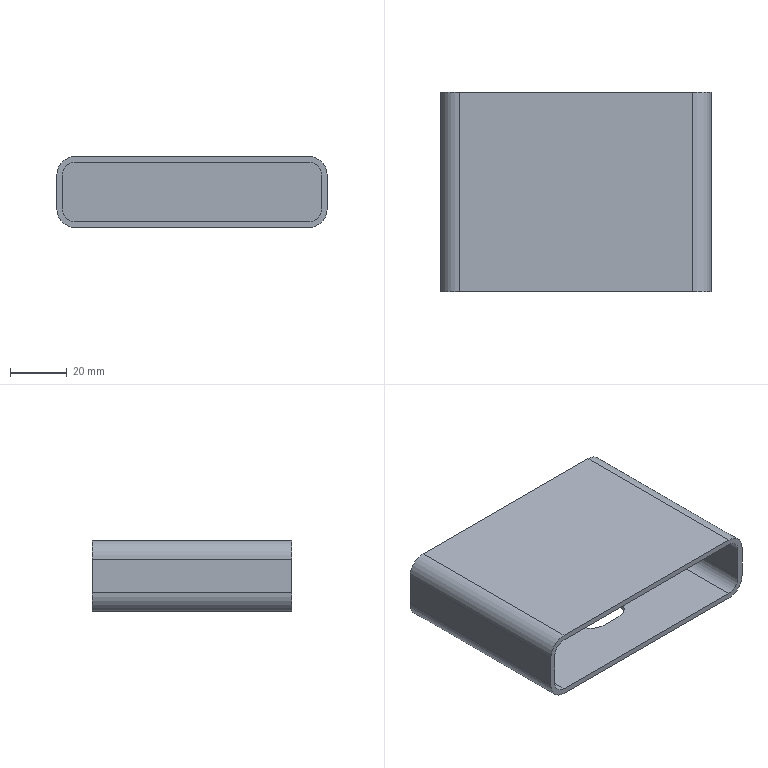Part | STEP file | Guide wheel mechanism revised.sldasm-Part-312 | 1 solid | 24 faces | box 95 x 70 x 25 mm | volume 34478 mm3 | plane 13 | cylinder 11 | commonest cylinder face diameters 9.083 x4 13.083 x4 13 x3
STEP:
#1=CARTESIAN_POINT('',(-10.173,-108.64,-53.));
#2=VERTEX_POINT('',#1);
#3=CARTESIAN_POINT('',(-3.673,-102.14,-53.));
#4=VERTEX_POINT('',#3);
#5=CARTESIAN_POINT('',(-3.673,-108.64,-53.));
#6=DIRECTION('',(0.,0.,-1.));
#7=DIRECTION('',(1.,0.,0.));
#8=AXIS2_PLACEMENT_3D('',#5,#6,#7);
#9=CIRCLE('',#8,6.5);
#10=EDGE_CURVE('',#2,#4,#9,.T.);
#11=ORIENTED_EDGE('',*,*,#10,.F.);
#12=CARTESIAN_POINT('',(-10.173,-108.64,-55.));
#13=VERTEX_POINT('',#12);
#14=CARTESIAN_POINT('',(-10.173,-108.64,0.001));
#15=DIRECTION('',(0.,0.,-1.));
#16=VECTOR('',#15,1000.);
#17=LINE('',#14,#16);
#18=EDGE_CURVE('',#2,#13,#17,.T.);
#19=ORIENTED_EDGE('',*,*,#18,.T.);
#20=CARTESIAN_POINT('',(-3.673,-102.14,-55.));
#21=VERTEX_POINT('',#20);
#22=CARTESIAN_POINT('',(-3.673,-108.64,-55.));
#23=DIRECTION('',(0.,0.,-1.));
#24=DIRECTION('',(-1.,0.,0.));
#25=AXIS2_PLACEMENT_3D('',#22,#23,#24);
#26=CIRCLE('',#25,6.5);
#27=EDGE_CURVE('',#13,#21,#26,.T.);
#28=ORIENTED_EDGE('',*,*,#27,.T.);
#29=CARTESIAN_POINT('',(-3.673,-102.14,0.001));
#30=DIRECTION('',(0.,0.,-1.));
#31=VECTOR('',#30,1000.);
#32=LINE('',#29,#31);
#33=EDGE_CURVE('',#4,#21,#32,.T.);
#34=ORIENTED_EDGE('',*,*,#33,.F.);
#35=EDGE_LOOP('',(#11,#19,#28,#34));
#36=FACE_OUTER_BOUND('',#35,.T.);
#37=CARTESIAN_POINT('',(-3.673,-108.64,0.001));
#38=DIRECTION('',(0.,0.,-1.));
#39=DIRECTION('',(-1.,0.,0.));
#40=AXIS2_PLACEMENT_3D('',#37,#38,#39);
#41=CYLINDRICAL_SURFACE('',#40,6.5);
#42=ADVANCED_FACE('',(#36),#41,.F.);
#43=CARTESIAN_POINT('',(-47.5,-132.5,-48.458));
#44=VERTEX_POINT('',#43);
#45=CARTESIAN_POINT('',(-40.958,-132.5,-55.));
#46=VERTEX_POINT('',#45);
#47=CARTESIAN_POINT('',(-40.958,-132.5,-48.458));
#48=DIRECTION('',(0.,-1.,0.));
#49=DIRECTION('',(0.,0.,1.));
#50=AXIS2_PLACEMENT_3D('',#47,#48,#49);
#51=CIRCLE('',#50,6.542);
#52=EDGE_CURVE('',#44,#46,#51,.T.);
#53=ORIENTED_EDGE('',*,*,#52,.T.);
#54=CARTESIAN_POINT('',(40.958,-132.5,-55.));
#55=VERTEX_POINT('',#54);
#56=CARTESIAN_POINT('',(-40.958,-132.5,-55.));
#57=DIRECTION('',(1.,0.,0.));
#58=VECTOR('',#57,1000.);
#59=LINE('',#56,#58);
#60=EDGE_CURVE('',#46,#55,#59,.T.);
#61=ORIENTED_EDGE('',*,*,#60,.T.);
#62=CARTESIAN_POINT('',(47.5,-132.5,-48.458));
#63=VERTEX_POINT('',#62);
#64=CARTESIAN_POINT('',(40.958,-132.5,-48.458));
#65=DIRECTION('',(0.,-1.,0.));
#66=DIRECTION('',(0.,0.,-1.));
#67=AXIS2_PLACEMENT_3D('',#64,#65,#66);
#68=CIRCLE('',#67,6.542);
#69=EDGE_CURVE('',#55,#63,#68,.T.);
#70=ORIENTED_EDGE('',*,*,#69,.T.);
#71=CARTESIAN_POINT('',(47.5,-132.5,-36.542));
#72=VERTEX_POINT('',#71);
#73=CARTESIAN_POINT('',(47.5,-132.5,-36.542));
#74=DIRECTION('',(0.,0.,1.));
#75=VECTOR('',#74,1000.);
#76=LINE('',#73,#75);
#77=EDGE_CURVE('',#63,#72,#76,.T.);
#78=ORIENTED_EDGE('',*,*,#77,.T.);
#79=CARTESIAN_POINT('',(40.958,-132.5,-30.));
#80=VERTEX_POINT('',#79);
#81=CARTESIAN_POINT('',(40.958,-132.5,-36.542));
#82=DIRECTION('',(0.,-1.,0.));
#83=DIRECTION('',(0.,0.,-1.));
#84=AXIS2_PLACEMENT_3D('',#81,#82,#83);
#85=CIRCLE('',#84,6.542);
#86=EDGE_CURVE('',#72,#80,#85,.T.);
#87=ORIENTED_EDGE('',*,*,#86,.T.);
#88=CARTESIAN_POINT('',(-40.958,-132.5,-30.));
#89=VERTEX_POINT('',#88);
#90=CARTESIAN_POINT('',(-40.958,-132.5,-30.));
#91=DIRECTION('',(-1.,0.,0.));
#92=VECTOR('',#91,1000.);
#93=LINE('',#90,#92);
#94=EDGE_CURVE('',#80,#89,#93,.T.);
#95=ORIENTED_EDGE('',*,*,#94,.T.);
#96=CARTESIAN_POINT('',(-47.5,-132.5,-36.542));
#97=VERTEX_POINT('',#96);
#98=CARTESIAN_POINT('',(-40.958,-132.5,-36.542));
#99=DIRECTION('',(0.,-1.,0.));
#100=DIRECTION('',(0.,0.,1.));
#101=AXIS2_PLACEMENT_3D('',#98,#99,#100);
#102=CIRCLE('',#101,6.542);
#103=EDGE_CURVE('',#89,#97,#102,.T.);
#104=ORIENTED_EDGE('',*,*,#103,.T.);
#105=CARTESIAN_POINT('',(-47.5,-132.5,-36.542));
#106=DIRECTION('',(0.,0.,-1.));
#107=VECTOR('',#106,1000.);
#108=LINE('',#105,#107);
#109=EDGE_CURVE('',#97,#44,#108,.T.);
#110=ORIENTED_EDGE('',*,*,#109,.T.);
#111=EDGE_LOOP('',(#53,#61,#70,#78,#87,#95,#104,#110));
#112=FACE_OUTER_BOUND('',#111,.T.);
#113=CARTESIAN_POINT('',(-45.5,-132.5,-48.458));
#114=VERTEX_POINT('',#113);
#115=CARTESIAN_POINT('',(-40.958,-132.5,-53.));
#116=VERTEX_POINT('',#115);
#117=CARTESIAN_POINT('',(-40.958,-132.5,-48.458));
#118=DIRECTION('',(0.,-1.,0.));
#119=DIRECTION('',(0.,0.,1.));
#120=AXIS2_PLACEMENT_3D('',#117,#118,#119);
#121=CIRCLE('',#120,4.542);
#122=EDGE_CURVE('',#114,#116,#121,.T.);
#123=ORIENTED_EDGE('',*,*,#122,.F.);
#124=CARTESIAN_POINT('',(-45.5,-132.5,-36.542));
#125=VERTEX_POINT('',#124);
#126=CARTESIAN_POINT('',(-45.5,-132.5,-48.458));
#127=DIRECTION('',(0.,0.,-1.));
#128=VECTOR('',#127,1000.);
#129=LINE('',#126,#128);
#130=EDGE_CURVE('',#125,#114,#129,.T.);
#131=ORIENTED_EDGE('',*,*,#130,.F.);
#132=CARTESIAN_POINT('',(-40.958,-132.5,-32.));
#133=VERTEX_POINT('',#132);
#134=CARTESIAN_POINT('',(-40.958,-132.5,-36.542));
#135=DIRECTION('',(0.,-1.,0.));
#136=DIRECTION('',(0.,0.,1.));
#137=AXIS2_PLACEMENT_3D('',#134,#135,#136);
#138=CIRCLE('',#137,4.542);
#139=EDGE_CURVE('',#133,#125,#138,.T.);
#140=ORIENTED_EDGE('',*,*,#139,.F.);
#141=CARTESIAN_POINT('',(40.958,-132.5,-32.));
#142=VERTEX_POINT('',#141);
#143=CARTESIAN_POINT('',(-40.958,-132.5,-32.));
#144=DIRECTION('',(-1.,0.,0.));
#145=VECTOR('',#144,1000.);
#146=LINE('',#143,#145);
#147=EDGE_CURVE('',#142,#133,#146,.T.);
#148=ORIENTED_EDGE('',*,*,#147,.F.);
#149=CARTESIAN_POINT('',(45.5,-132.5,-36.542));
#150=VERTEX_POINT('',#149);
#151=CARTESIAN_POINT('',(40.958,-132.5,-36.542));
#152=DIRECTION('',(0.,-1.,0.));
#153=DIRECTION('',(0.,0.,1.));
#154=AXIS2_PLACEMENT_3D('',#151,#152,#153);
#155=CIRCLE('',#154,4.542);
#156=EDGE_CURVE('',#150,#142,#155,.T.);
#157=ORIENTED_EDGE('',*,*,#156,.F.);
#158=CARTESIAN_POINT('',(45.5,-132.5,-48.458));
#159=VERTEX_POINT('',#158);
#160=CARTESIAN_POINT('',(45.5,-132.5,-48.458));
#161=DIRECTION('',(0.,0.,1.));
#162=VECTOR('',#161,1000.);
#163=LINE('',#160,#162);
#164=EDGE_CURVE('',#159,#150,#163,.T.);
#165=ORIENTED_EDGE('',*,*,#164,.F.);
#166=CARTESIAN_POINT('',(40.958,-132.5,-53.));
#167=VERTEX_POINT('',#166);
#168=CARTESIAN_POINT('',(40.958,-132.5,-48.458));
#169=DIRECTION('',(0.,-1.,0.));
#170=DIRECTION('',(0.,0.,1.));
#171=AXIS2_PLACEMENT_3D('',#168,#169,#170);
#172=CIRCLE('',#171,4.542);
#173=EDGE_CURVE('',#167,#159,#172,.T.);
#174=ORIENTED_EDGE('',*,*,#173,.F.);
#175=CARTESIAN_POINT('',(-40.958,-132.5,-53.));
#176=DIRECTION('',(1.,0.,0.));
#177=VECTOR('',#176,1000.);
#178=LINE('',#175,#177);
#179=EDGE_CURVE('',#116,#167,#178,.T.);
#180=ORIENTED_EDGE('',*,*,#179,.F.);
#181=EDGE_LOOP('',(#123,#131,#140,#148,#157,#165,#174,#180));
#182=FACE_BOUND('',#181,.T.);
#183=CARTESIAN_POINT('',(-40.958,-132.5,-48.458));
#184=DIRECTION('',(0.,1.,0.));
#185=DIRECTION('',(0.,0.,1.));
#186=AXIS2_PLACEMENT_3D('',#183,#184,#185);
#187=PLANE('',#186);
#188=ADVANCED_FACE('',(#112,#182),#187,.F.);
#189=CARTESIAN_POINT('',(-47.5,-62.5,-48.458));
#190=VERTEX_POINT('',#189);
#191=CARTESIAN_POINT('',(-40.958,-62.5,-55.));
#192=VERTEX_POINT('',#191);
#193=CARTESIAN_POINT('',(-40.958,-62.5,-48.458));
#194=DIRECTION('',(0.,-1.,0.));
#195=DIRECTION('',(0.,0.,1.));
#196=AXIS2_PLACEMENT_3D('',#193,#194,#195);
#197=CIRCLE('',#196,6.542);
#198=EDGE_CURVE('',#190,#192,#197,.T.);
#199=ORIENTED_EDGE('',*,*,#198,.T.);
#200=CARTESIAN_POINT('',(-40.958,-132.5,-55.));
#201=DIRECTION('',(0.,1.,0.));
#202=VECTOR('',#201,1000.);
#203=LINE('',#200,#202);
#204=EDGE_CURVE('',#46,#192,#203,.T.);
#205=ORIENTED_EDGE('',*,*,#204,.F.);
#206=ORIENTED_EDGE('',*,*,#52,.F.);
#207=CARTESIAN_POINT('',(-47.5,-132.5,-48.458));
#208=DIRECTION('',(0.,1.,0.));
#209=VECTOR('',#208,1000.);
#210=LINE('',#207,#209);
#211=EDGE_CURVE('',#44,#190,#210,.T.);
#212=ORIENTED_EDGE('',*,*,#211,.T.);
#213=EDGE_LOOP('',(#199,#205,#206,#212));
#214=FACE_OUTER_BOUND('',#213,.T.);
#215=CARTESIAN_POINT('',(-40.958,-132.5,-48.458));
#216=DIRECTION('',(0.,1.,0.));
#217=DIRECTION('',(0.,0.,1.));
#218=AXIS2_PLACEMENT_3D('',#215,#216,#217);
#219=CYLINDRICAL_SURFACE('',#218,6.542);
#220=ADVANCED_FACE('',(#214),#219,.T.);
#221=CARTESIAN_POINT('',(3.673,-115.14,-55.));
#222=VERTEX_POINT('',#221);
#223=CARTESIAN_POINT('',(-3.673,-115.14,-55.));
#224=VERTEX_POINT('',#223);
#225=CARTESIAN_POINT('',(3.673,-115.14,-55.));
#226=DIRECTION('',(-1.,0.,0.));
#227=VECTOR('',#226,1000.);
#228=LINE('',#225,#227);
#229=EDGE_CURVE('',#222,#224,#228,.T.);
#230=ORIENTED_EDGE('',*,*,#229,.F.);
#231=CARTESIAN_POINT('',(3.673,-102.14,-55.));
#232=VERTEX_POINT('',#231);
#233=CARTESIAN_POINT('',(3.673,-108.64,-55.));
#234=DIRECTION('',(0.,0.,-1.));
#235=DIRECTION('',(-1.,0.,0.));
#236=AXIS2_PLACEMENT_3D('',#233,#234,#235);
#237=CIRCLE('',#236,6.5);
#238=EDGE_CURVE('',#232,#222,#237,.T.);
#239=ORIENTED_EDGE('',*,*,#238,.F.);
#240=CARTESIAN_POINT('',(3.673,-102.14,-55.));
#241=DIRECTION('',(1.,0.,0.));
#242=VECTOR('',#241,1000.);
#243=LINE('',#240,#242);
#244=EDGE_CURVE('',#21,#232,#243,.T.);
#245=ORIENTED_EDGE('',*,*,#244,.F.);
#246=ORIENTED_EDGE('',*,*,#27,.F.);
#247=CARTESIAN_POINT('',(-3.673,-108.64,-55.));
#248=DIRECTION('',(0.,0.,-1.));
#249=DIRECTION('',(-1.,0.,0.));
#250=AXIS2_PLACEMENT_3D('',#247,#248,#249);
#251=CIRCLE('',#250,6.5);
#252=EDGE_CURVE('',#224,#13,#251,.T.);
#253=ORIENTED_EDGE('',*,*,#252,.F.);
#254=EDGE_LOOP('',(#230,#239,#245,#246,#253));
#255=FACE_BOUND('',#254,.T.);
#256=CARTESIAN_POINT('',(40.958,-62.5,-55.));
#257=VERTEX_POINT('',#256);
#258=CARTESIAN_POINT('',(-40.958,-62.5,-55.));
#259=DIRECTION('',(1.,0.,0.));
#260=VECTOR('',#259,1000.);
#261=LINE('',#258,#260);
#262=EDGE_CURVE('',#192,#257,#261,.T.);
#263=ORIENTED_EDGE('',*,*,#262,.T.);
#264=CARTESIAN_POINT('',(40.958,-132.5,-55.));
#265=DIRECTION('',(0.,1.,0.));
#266=VECTOR('',#265,1000.);
#267=LINE('',#264,#266);
#268=EDGE_CURVE('',#55,#257,#267,.T.);
#269=ORIENTED_EDGE('',*,*,#268,.F.);
#270=ORIENTED_EDGE('',*,*,#60,.F.);
#271=ORIENTED_EDGE('',*,*,#204,.T.);
#272=EDGE_LOOP('',(#263,#269,#270,#271));
#273=FACE_OUTER_BOUND('',#272,.T.);
#274=CARTESIAN_POINT('',(-40.958,-132.5,-55.));
#275=DIRECTION('',(0.,0.,1.));
#276=DIRECTION('',(1.,0.,0.));
#277=AXIS2_PLACEMENT_3D('',#274,#275,#276);
#278=PLANE('',#277);
#279=ADVANCED_FACE('',(#255,#273),#278,.F.);
#280=CARTESIAN_POINT('',(47.5,-62.5,-48.458));
#281=VERTEX_POINT('',#280);
#282=CARTESIAN_POINT('',(40.958,-62.5,-48.458));
#283=DIRECTION('',(0.,-1.,0.));
#284=DIRECTION('',(0.,0.,-1.));
#285=AXIS2_PLACEMENT_3D('',#282,#283,#284);
#286=CIRCLE('',#285,6.542);
#287=EDGE_CURVE('',#257,#281,#286,.T.);
#288=ORIENTED_EDGE('',*,*,#287,.T.);
#289=CARTESIAN_POINT('',(47.5,-132.5,-48.458));
#290=DIRECTION('',(0.,1.,0.));
#291=VECTOR('',#290,1000.);
#292=LINE('',#289,#291);
#293=EDGE_CURVE('',#63,#281,#292,.T.);
#294=ORIENTED_EDGE('',*,*,#293,.F.);
#295=ORIENTED_EDGE('',*,*,#69,.F.);
#296=ORIENTED_EDGE('',*,*,#268,.T.);
#297=EDGE_LOOP('',(#288,#294,#295,#296));
#298=FACE_OUTER_BOUND('',#297,.T.);
#299=CARTESIAN_POINT('',(40.958,-132.5,-48.458));
#300=DIRECTION('',(0.,1.,0.));
#301=DIRECTION('',(0.,0.,1.));
#302=AXIS2_PLACEMENT_3D('',#299,#300,#301);
#303=CYLINDRICAL_SURFACE('',#302,6.542);
#304=ADVANCED_FACE('',(#298),#303,.T.);
#305=CARTESIAN_POINT('',(47.5,-62.5,-36.542));
#306=VERTEX_POINT('',#305);
#307=CARTESIAN_POINT('',(47.5,-62.5,-36.542));
#308=DIRECTION('',(0.,0.,1.));
#309=VECTOR('',#308,1000.);
#310=LINE('',#307,#309);
#311=EDGE_CURVE('',#281,#306,#310,.T.);
#312=ORIENTED_EDGE('',*,*,#311,.T.);
#313=CARTESIAN_POINT('',(47.5,-132.5,-36.542));
#314=DIRECTION('',(0.,1.,0.));
#315=VECTOR('',#314,1000.);
#316=LINE('',#313,#315);
#317=EDGE_CURVE('',#72,#306,#316,.T.);
#318=ORIENTED_EDGE('',*,*,#317,.F.);
#319=ORIENTED_EDGE('',*,*,#77,.F.);
#320=ORIENTED_EDGE('',*,*,#293,.T.);
#321=EDGE_LOOP('',(#312,#318,#319,#320));
#322=FACE_OUTER_BOUND('',#321,.T.);
#323=CARTESIAN_POINT('',(47.5,-132.5,-36.542));
#324=DIRECTION('',(-1.,0.,0.));
#325=DIRECTION('',(0.,0.,1.));
#326=AXIS2_PLACEMENT_3D('',#323,#324,#325);
#327=PLANE('',#326);
#328=ADVANCED_FACE('',(#322),#327,.F.);
#329=CARTESIAN_POINT('',(40.958,-62.5,-30.));
#330=VERTEX_POINT('',#329);
#331=CARTESIAN_POINT('',(40.958,-62.5,-36.542));
#332=DIRECTION('',(0.,-1.,0.));
#333=DIRECTION('',(0.,0.,-1.));
#334=AXIS2_PLACEMENT_3D('',#331,#332,#333);
#335=CIRCLE('',#334,6.542);
#336=EDGE_CURVE('',#306,#330,#335,.T.);
#337=ORIENTED_EDGE('',*,*,#336,.T.);
#338=CARTESIAN_POINT('',(40.958,-132.5,-30.));
#339=DIRECTION('',(0.,1.,0.));
#340=VECTOR('',#339,1000.);
#341=LINE('',#338,#340);
#342=EDGE_CURVE('',#80,#330,#341,.T.);
#343=ORIENTED_EDGE('',*,*,#342,.F.);
#344=ORIENTED_EDGE('',*,*,#86,.F.);
#345=ORIENTED_EDGE('',*,*,#317,.T.);
#346=EDGE_LOOP('',(#337,#343,#344,#345));
#347=FACE_OUTER_BOUND('',#346,.T.);
#348=CARTESIAN_POINT('',(40.958,-132.5,-36.542));
#349=DIRECTION('',(0.,1.,0.));
#350=DIRECTION('',(0.,0.,1.));
#351=AXIS2_PLACEMENT_3D('',#348,#349,#350);
#352=CYLINDRICAL_SURFACE('',#351,6.542);
#353=ADVANCED_FACE('',(#347),#352,.T.);
#354=CARTESIAN_POINT('',(-40.958,-62.5,-30.));
#355=VERTEX_POINT('',#354);
#356=CARTESIAN_POINT('',(-40.958,-62.5,-30.));
#357=DIRECTION('',(-1.,0.,0.));
#358=VECTOR('',#357,1000.);
#359=LINE('',#356,#358);
#360=EDGE_CURVE('',#330,#355,#359,.T.);
#361=ORIENTED_EDGE('',*,*,#360,.T.);
#362=CARTESIAN_POINT('',(-40.958,-132.5,-30.));
#363=DIRECTION('',(0.,1.,0.));
#364=VECTOR('',#363,1000.);
#365=LINE('',#362,#364);
#366=EDGE_CURVE('',#89,#355,#365,.T.);
#367=ORIENTED_EDGE('',*,*,#366,.F.);
#368=ORIENTED_EDGE('',*,*,#94,.F.);
#369=ORIENTED_EDGE('',*,*,#342,.T.);
#370=EDGE_LOOP('',(#361,#367,#368,#369));
#371=FACE_OUTER_BOUND('',#370,.T.);
#372=CARTESIAN_POINT('',(-40.958,-132.5,-30.));
#373=DIRECTION('',(0.,0.,-1.));
#374=DIRECTION('',(-1.,0.,0.));
#375=AXIS2_PLACEMENT_3D('',#372,#373,#374);
#376=PLANE('',#375);
#377=ADVANCED_FACE('',(#371),#376,.F.);
#378=CARTESIAN_POINT('',(-47.5,-62.5,-36.542));
#379=VERTEX_POINT('',#378);
#380=CARTESIAN_POINT('',(-40.958,-62.5,-36.542));
#381=DIRECTION('',(0.,-1.,0.));
#382=DIRECTION('',(0.,0.,1.));
#383=AXIS2_PLACEMENT_3D('',#380,#381,#382);
#384=CIRCLE('',#383,6.542);
#385=EDGE_CURVE('',#355,#379,#384,.T.);
#386=ORIENTED_EDGE('',*,*,#385,.T.);
#387=CARTESIAN_POINT('',(-47.5,-132.5,-36.542));
#388=DIRECTION('',(0.,1.,0.));
#389=VECTOR('',#388,1000.);
#390=LINE('',#387,#389);
#391=EDGE_CURVE('',#97,#379,#390,.T.);
#392=ORIENTED_EDGE('',*,*,#391,.F.);
#393=ORIENTED_EDGE('',*,*,#103,.F.);
#394=ORIENTED_EDGE('',*,*,#366,.T.);
#395=EDGE_LOOP('',(#386,#392,#393,#394));
#396=FACE_OUTER_BOUND('',#395,.T.);
#397=CARTESIAN_POINT('',(-40.958,-132.5,-36.542));
#398=DIRECTION('',(0.,1.,0.));
#399=DIRECTION('',(0.,0.,1.));
#400=AXIS2_PLACEMENT_3D('',#397,#398,#399);
#401=CYLINDRICAL_SURFACE('',#400,6.542);
#402=ADVANCED_FACE('',(#396),#401,.T.);
#403=CARTESIAN_POINT('',(-47.5,-62.5,-36.542));
#404=DIRECTION('',(0.,0.,-1.));
#405=VECTOR('',#404,1000.);
#406=LINE('',#403,#405);
#407=EDGE_CURVE('',#379,#190,#406,.T.);
#408=ORIENTED_EDGE('',*,*,#407,.T.);
#409=ORIENTED_EDGE('',*,*,#211,.F.);
#410=ORIENTED_EDGE('',*,*,#109,.F.);
#411=ORIENTED_EDGE('',*,*,#391,.T.);
#412=EDGE_LOOP('',(#408,#409,#410,#411));
#413=FACE_OUTER_BOUND('',#412,.T.);
#414=CARTESIAN_POINT('',(-47.5,-132.5,-36.542));
#415=DIRECTION('',(1.,0.,0.));
#416=DIRECTION('',(0.,0.,-1.));
#417=AXIS2_PLACEMENT_3D('',#414,#415,#416);
#418=PLANE('',#417);
#419=ADVANCED_FACE('',(#413),#418,.F.);
#420=ORIENTED_EDGE('',*,*,#198,.F.);
#421=ORIENTED_EDGE('',*,*,#407,.F.);
#422=ORIENTED_EDGE('',*,*,#385,.F.);
#423=ORIENTED_EDGE('',*,*,#360,.F.);
#424=ORIENTED_EDGE('',*,*,#336,.F.);
#425=ORIENTED_EDGE('',*,*,#311,.F.);
#426=ORIENTED_EDGE('',*,*,#287,.F.);
#427=ORIENTED_EDGE('',*,*,#262,.F.);
#428=EDGE_LOOP('',(#420,#421,#422,#423,#424,#425,#426,#427));
#429=FACE_OUTER_BOUND('',#428,.T.);
#430=CARTESIAN_POINT('',(-40.958,-62.5,-48.458));
#431=DIRECTION('',(0.,1.,0.));
#432=DIRECTION('',(0.,0.,1.));
#433=AXIS2_PLACEMENT_3D('',#430,#431,#432);
#434=PLANE('',#433);
#435=ADVANCED_FACE('',(#429),#434,.T.);
#436=CARTESIAN_POINT('',(-45.5,-64.5,-48.458));
#437=VERTEX_POINT('',#436);
#438=CARTESIAN_POINT('',(-40.958,-64.5,-53.));
#439=VERTEX_POINT('',#438);
#440=CARTESIAN_POINT('',(-40.958,-64.5,-48.458));
#441=DIRECTION('',(0.,-1.,0.));
#442=DIRECTION('',(0.,0.,1.));
#443=AXIS2_PLACEMENT_3D('',#440,#441,#442);
#444=CIRCLE('',#443,4.542);
#445=EDGE_CURVE('',#437,#439,#444,.T.);
#446=ORIENTED_EDGE('',*,*,#445,.F.);
#447=CARTESIAN_POINT('',(-45.5,-132.5,-48.458));
#448=DIRECTION('',(0.,1.,0.));
#449=VECTOR('',#448,1000.);
#450=LINE('',#447,#449);
#451=EDGE_CURVE('',#114,#437,#450,.T.);
#452=ORIENTED_EDGE('',*,*,#451,.F.);
#453=ORIENTED_EDGE('',*,*,#122,.T.);
#454=CARTESIAN_POINT('',(-40.958,-132.5,-53.));
#455=DIRECTION('',(0.,1.,0.));
#456=VECTOR('',#455,1000.);
#457=LINE('',#454,#456);
#458=EDGE_CURVE('',#116,#439,#457,.T.);
#459=ORIENTED_EDGE('',*,*,#458,.T.);
#460=EDGE_LOOP('',(#446,#452,#453,#459));
#461=FACE_OUTER_BOUND('',#460,.T.);
#462=CARTESIAN_POINT('',(-40.958,-132.5,-48.458));
#463=DIRECTION('',(0.,1.,0.));
#464=DIRECTION('',(0.,0.,1.));
#465=AXIS2_PLACEMENT_3D('',#462,#463,#464);
#466=CYLINDRICAL_SURFACE('',#465,4.542);
#467=ADVANCED_FACE('',(#461),#466,.F.);
#468=CARTESIAN_POINT('',(3.673,-102.14,-53.));
#469=VERTEX_POINT('',#468);
#470=CARTESIAN_POINT('',(3.673,-115.14,-53.));
#471=VERTEX_POINT('',#470);
#472=CARTESIAN_POINT('',(3.673,-108.64,-53.));
#473=DIRECTION('',(0.,0.,-1.));
#474=DIRECTION('',(1.,0.,0.));
#475=AXIS2_PLACEMENT_3D('',#472,#473,#474);
#476=CIRCLE('',#475,6.5);
#477=EDGE_CURVE('',#469,#471,#476,.T.);
#478=ORIENTED_EDGE('',*,*,#477,.T.);
#479=CARTESIAN_POINT('',(-3.673,-115.14,-53.));
#480=VERTEX_POINT('',#479);
#481=CARTESIAN_POINT('',(3.673,-115.14,-53.));
#482=DIRECTION('',(-1.,0.,0.));
#483=VECTOR('',#482,1000.);
#484=LINE('',#481,#483);
#485=EDGE_CURVE('',#471,#480,#484,.T.);
#486=ORIENTED_EDGE('',*,*,#485,.T.);
#487=CARTESIAN_POINT('',(-3.673,-108.64,-53.));
#488=DIRECTION('',(0.,0.,-1.));
#489=DIRECTION('',(1.,0.,0.));
#490=AXIS2_PLACEMENT_3D('',#487,#488,#489);
#491=CIRCLE('',#490,6.5);
#492=EDGE_CURVE('',#480,#2,#491,.T.);
#493=ORIENTED_EDGE('',*,*,#492,.T.);
#494=ORIENTED_EDGE('',*,*,#10,.T.);
#495=CARTESIAN_POINT('',(3.673,-102.14,-53.));
#496=DIRECTION('',(1.,0.,0.));
#497=VECTOR('',#496,1000.);
#498=LINE('',#495,#497);
#499=EDGE_CURVE('',#4,#469,#498,.T.);
#500=ORIENTED_EDGE('',*,*,#499,.T.);
#501=EDGE_LOOP('',(#478,#486,#493,#494,#500));
#502=FACE_BOUND('',#501,.T.);
#503=CARTESIAN_POINT('',(40.958,-64.5,-53.));
#504=VERTEX_POINT('',#503);
#505=CARTESIAN_POINT('',(-40.958,-64.5,-53.));
#506=DIRECTION('',(1.,0.,0.));
#507=VECTOR('',#506,1000.);
#508=LINE('',#505,#507);
#509=EDGE_CURVE('',#439,#504,#508,.T.);
#510=ORIENTED_EDGE('',*,*,#509,.F.);
#511=ORIENTED_EDGE('',*,*,#458,.F.);
#512=ORIENTED_EDGE('',*,*,#179,.T.);
#513=CARTESIAN_POINT('',(40.958,-132.5,-53.));
#514=DIRECTION('',(0.,1.,0.));
#515=VECTOR('',#514,1000.);
#516=LINE('',#513,#515);
#517=EDGE_CURVE('',#167,#504,#516,.T.);
#518=ORIENTED_EDGE('',*,*,#517,.T.);
#519=EDGE_LOOP('',(#510,#511,#512,#518));
#520=FACE_OUTER_BOUND('',#519,.T.);
#521=CARTESIAN_POINT('',(-40.958,-132.5,-53.));
#522=DIRECTION('',(0.,0.,1.));
#523=DIRECTION('',(1.,0.,0.));
#524=AXIS2_PLACEMENT_3D('',#521,#522,#523);
#525=PLANE('',#524);
#526=ADVANCED_FACE('',(#502,#520),#525,.T.);
#527=CARTESIAN_POINT('',(45.5,-64.5,-48.458));
#528=VERTEX_POINT('',#527);
#529=CARTESIAN_POINT('',(40.958,-64.5,-48.458));
#530=DIRECTION('',(0.,-1.,0.));
#531=DIRECTION('',(0.,0.,1.));
#532=AXIS2_PLACEMENT_3D('',#529,#530,#531);
#533=CIRCLE('',#532,4.542);
#534=EDGE_CURVE('',#504,#528,#533,.T.);
#535=ORIENTED_EDGE('',*,*,#534,.F.);
#536=ORIENTED_EDGE('',*,*,#517,.F.);
#537=ORIENTED_EDGE('',*,*,#173,.T.);
#538=CARTESIAN_POINT('',(45.5,-132.5,-48.458));
#539=DIRECTION('',(0.,1.,0.));
#540=VECTOR('',#539,1000.);
#541=LINE('',#538,#540);
#542=EDGE_CURVE('',#159,#528,#541,.T.);
#543=ORIENTED_EDGE('',*,*,#542,.T.);
#544=EDGE_LOOP('',(#535,#536,#537,#543));
#545=FACE_OUTER_BOUND('',#544,.T.);
#546=CARTESIAN_POINT('',(40.958,-132.5,-48.458));
#547=DIRECTION('',(0.,1.,0.));
#548=DIRECTION('',(0.,0.,1.));
#549=AXIS2_PLACEMENT_3D('',#546,#547,#548);
#550=CYLINDRICAL_SURFACE('',#549,4.542);
#551=ADVANCED_FACE('',(#545),#550,.F.);
#552=CARTESIAN_POINT('',(45.5,-64.5,-36.542));
#553=VERTEX_POINT('',#552);
#554=CARTESIAN_POINT('',(45.5,-64.5,-48.458));
#555=DIRECTION('',(0.,0.,1.));
#556=VECTOR('',#555,1000.);
#557=LINE('',#554,#556);
#558=EDGE_CURVE('',#528,#553,#557,.T.);
#559=ORIENTED_EDGE('',*,*,#558,.F.);
#560=ORIENTED_EDGE('',*,*,#542,.F.);
#561=ORIENTED_EDGE('',*,*,#164,.T.);
#562=CARTESIAN_POINT('',(45.5,-132.5,-36.542));
#563=DIRECTION('',(0.,1.,0.));
#564=VECTOR('',#563,1000.);
#565=LINE('',#562,#564);
#566=EDGE_CURVE('',#150,#553,#565,.T.);
#567=ORIENTED_EDGE('',*,*,#566,.T.);
#568=EDGE_LOOP('',(#559,#560,#561,#567));
#569=FACE_OUTER_BOUND('',#568,.T.);
#570=CARTESIAN_POINT('',(45.5,-132.5,-36.542));
#571=DIRECTION('',(-1.,0.,0.));
#572=DIRECTION('',(0.,0.,1.));
#573=AXIS2_PLACEMENT_3D('',#570,#571,#572);
#574=PLANE('',#573);
#575=ADVANCED_FACE('',(#569),#574,.T.);
#576=CARTESIAN_POINT('',(40.958,-64.5,-32.));
#577=VERTEX_POINT('',#576);
#578=CARTESIAN_POINT('',(40.958,-64.5,-36.542));
#579=DIRECTION('',(0.,-1.,0.));
#580=DIRECTION('',(0.,0.,1.));
#581=AXIS2_PLACEMENT_3D('',#578,#579,#580);
#582=CIRCLE('',#581,4.542);
#583=EDGE_CURVE('',#553,#577,#582,.T.);
#584=ORIENTED_EDGE('',*,*,#583,.F.);
#585=ORIENTED_EDGE('',*,*,#566,.F.);
#586=ORIENTED_EDGE('',*,*,#156,.T.);
#587=CARTESIAN_POINT('',(40.958,-132.5,-32.));
#588=DIRECTION('',(0.,1.,0.));
#589=VECTOR('',#588,1000.);
#590=LINE('',#587,#589);
#591=EDGE_CURVE('',#142,#577,#590,.T.);
#592=ORIENTED_EDGE('',*,*,#591,.T.);
#593=EDGE_LOOP('',(#584,#585,#586,#592));
#594=FACE_OUTER_BOUND('',#593,.T.);
#595=CARTESIAN_POINT('',(40.958,-132.5,-36.542));
#596=DIRECTION('',(0.,1.,0.));
#597=DIRECTION('',(0.,0.,1.));
#598=AXIS2_PLACEMENT_3D('',#595,#596,#597);
#599=CYLINDRICAL_SURFACE('',#598,4.542);
#600=ADVANCED_FACE('',(#594),#599,.F.);
#601=CARTESIAN_POINT('',(-40.958,-64.5,-32.));
#602=VERTEX_POINT('',#601);
#603=CARTESIAN_POINT('',(-40.958,-64.5,-32.));
#604=DIRECTION('',(-1.,0.,0.));
#605=VECTOR('',#604,1000.);
#606=LINE('',#603,#605);
#607=EDGE_CURVE('',#577,#602,#606,.T.);
#608=ORIENTED_EDGE('',*,*,#607,.F.);
#609=ORIENTED_EDGE('',*,*,#591,.F.);
#610=ORIENTED_EDGE('',*,*,#147,.T.);
#611=CARTESIAN_POINT('',(-40.958,-132.5,-32.));
#612=DIRECTION('',(0.,1.,0.));
#613=VECTOR('',#612,1000.);
#614=LINE('',#611,#613);
#615=EDGE_CURVE('',#133,#602,#614,.T.);
#616=ORIENTED_EDGE('',*,*,#615,.T.);
#617=EDGE_LOOP('',(#608,#609,#610,#616));
#618=FACE_OUTER_BOUND('',#617,.T.);
#619=CARTESIAN_POINT('',(-40.958,-132.5,-32.));
#620=DIRECTION('',(0.,0.,-1.));
#621=DIRECTION('',(-1.,0.,0.));
#622=AXIS2_PLACEMENT_3D('',#619,#620,#621);
#623=PLANE('',#622);
#624=ADVANCED_FACE('',(#618),#623,.T.);
#625=CARTESIAN_POINT('',(-45.5,-64.5,-36.542));
#626=VERTEX_POINT('',#625);
#627=CARTESIAN_POINT('',(-40.958,-64.5,-36.542));
#628=DIRECTION('',(0.,-1.,0.));
#629=DIRECTION('',(0.,0.,1.));
#630=AXIS2_PLACEMENT_3D('',#627,#628,#629);
#631=CIRCLE('',#630,4.542);
#632=EDGE_CURVE('',#602,#626,#631,.T.);
#633=ORIENTED_EDGE('',*,*,#632,.F.);
#634=ORIENTED_EDGE('',*,*,#615,.F.);
#635=ORIENTED_EDGE('',*,*,#139,.T.);
#636=CARTESIAN_POINT('',(-45.5,-132.5,-36.542));
#637=DIRECTION('',(0.,1.,0.));
#638=VECTOR('',#637,1000.);
#639=LINE('',#636,#638);
#640=EDGE_CURVE('',#125,#626,#639,.T.);
#641=ORIENTED_EDGE('',*,*,#640,.T.);
#642=EDGE_LOOP('',(#633,#634,#635,#641));
#643=FACE_OUTER_BOUND('',#642,.T.);
#644=CARTESIAN_POINT('',(-40.958,-132.5,-36.542));
#645=DIRECTION('',(0.,1.,0.));
#646=DIRECTION('',(0.,0.,1.));
#647=AXIS2_PLACEMENT_3D('',#644,#645,#646);
#648=CYLINDRICAL_SURFACE('',#647,4.542);
#649=ADVANCED_FACE('',(#643),#648,.F.);
#650=CARTESIAN_POINT('',(-45.5,-64.5,-48.458));
#651=DIRECTION('',(0.,0.,-1.));
#652=VECTOR('',#651,1000.);
#653=LINE('',#650,#652);
#654=EDGE_CURVE('',#626,#437,#653,.T.);
#655=ORIENTED_EDGE('',*,*,#654,.F.);
#656=ORIENTED_EDGE('',*,*,#640,.F.);
#657=ORIENTED_EDGE('',*,*,#130,.T.);
#658=ORIENTED_EDGE('',*,*,#451,.T.);
#659=EDGE_LOOP('',(#655,#656,#657,#658));
#660=FACE_OUTER_BOUND('',#659,.T.);
#661=CARTESIAN_POINT('',(-45.5,-132.5,-36.542));
#662=DIRECTION('',(1.,0.,0.));
#663=DIRECTION('',(0.,0.,-1.));
#664=AXIS2_PLACEMENT_3D('',#661,#662,#663);
#665=PLANE('',#664);
#666=ADVANCED_FACE('',(#660),#665,.T.);
#667=ORIENTED_EDGE('',*,*,#445,.T.);
#668=ORIENTED_EDGE('',*,*,#509,.T.);
#669=ORIENTED_EDGE('',*,*,#534,.T.);
#670=ORIENTED_EDGE('',*,*,#558,.T.);
#671=ORIENTED_EDGE('',*,*,#583,.T.);
#672=ORIENTED_EDGE('',*,*,#607,.T.);
#673=ORIENTED_EDGE('',*,*,#632,.T.);
#674=ORIENTED_EDGE('',*,*,#654,.T.);
#675=EDGE_LOOP('',(#667,#668,#669,#670,#671,#672,#673,#674));
#676=FACE_OUTER_BOUND('',#675,.T.);
#677=CARTESIAN_POINT('',(-40.958,-64.5,-48.458));
#678=DIRECTION('',(0.,1.,0.));
#679=DIRECTION('',(0.,0.,1.));
#680=AXIS2_PLACEMENT_3D('',#677,#678,#679);
#681=PLANE('',#680);
#682=ADVANCED_FACE('',(#676),#681,.F.);
#683=CARTESIAN_POINT('',(3.673,-102.14,0.001));
#684=DIRECTION('',(0.,0.,-1.));
#685=VECTOR('',#684,1000.);
#686=LINE('',#683,#685);
#687=EDGE_CURVE('',#469,#232,#686,.T.);
#688=ORIENTED_EDGE('',*,*,#687,.T.);
#689=ORIENTED_EDGE('',*,*,#238,.T.);
#690=CARTESIAN_POINT('',(3.673,-115.14,0.001));
#691=DIRECTION('',(0.,0.,-1.));
#692=VECTOR('',#691,1000.);
#693=LINE('',#690,#692);
#694=EDGE_CURVE('',#471,#222,#693,.T.);
#695=ORIENTED_EDGE('',*,*,#694,.F.);
#696=ORIENTED_EDGE('',*,*,#477,.F.);
#697=EDGE_LOOP('',(#688,#689,#695,#696));
#698=FACE_OUTER_BOUND('',#697,.T.);
#699=CARTESIAN_POINT('',(3.673,-108.64,0.001));
#700=DIRECTION('',(0.,0.,-1.));
#701=DIRECTION('',(-1.,0.,0.));
#702=AXIS2_PLACEMENT_3D('',#699,#700,#701);
#703=CYLINDRICAL_SURFACE('',#702,6.5);
#704=ADVANCED_FACE('',(#698),#703,.F.);
#705=ORIENTED_EDGE('',*,*,#33,.T.);
#706=ORIENTED_EDGE('',*,*,#244,.T.);
#707=ORIENTED_EDGE('',*,*,#687,.F.);
#708=ORIENTED_EDGE('',*,*,#499,.F.);
#709=EDGE_LOOP('',(#705,#706,#707,#708));
#710=FACE_OUTER_BOUND('',#709,.T.);
#711=CARTESIAN_POINT('',(3.673,-102.14,0.001));
#712=DIRECTION('',(0.,1.,0.));
#713=DIRECTION('',(0.,0.,1.));
#714=AXIS2_PLACEMENT_3D('',#711,#712,#713);
#715=PLANE('',#714);
#716=ADVANCED_FACE('',(#710),#715,.F.);
#717=ORIENTED_EDGE('',*,*,#18,.F.);
#718=ORIENTED_EDGE('',*,*,#492,.F.);
#719=CARTESIAN_POINT('',(-3.673,-115.14,0.001));
#720=DIRECTION('',(0.,0.,-1.));
#721=VECTOR('',#720,1000.);
#722=LINE('',#719,#721);
#723=EDGE_CURVE('',#480,#224,#722,.T.);
#724=ORIENTED_EDGE('',*,*,#723,.T.);
#725=ORIENTED_EDGE('',*,*,#252,.T.);
#726=EDGE_LOOP('',(#717,#718,#724,#725));
#727=FACE_OUTER_BOUND('',#726,.T.);
#728=CARTESIAN_POINT('',(-3.673,-108.64,0.001));
#729=DIRECTION('',(0.,0.,-1.));
#730=DIRECTION('',(-1.,0.,0.));
#731=AXIS2_PLACEMENT_3D('',#728,#729,#730);
#732=CYLINDRICAL_SURFACE('',#731,6.5);
#733=ADVANCED_FACE('',(#727),#732,.F.);
#734=ORIENTED_EDGE('',*,*,#694,.T.);
#735=ORIENTED_EDGE('',*,*,#229,.T.);
#736=ORIENTED_EDGE('',*,*,#723,.F.);
#737=ORIENTED_EDGE('',*,*,#485,.F.);
#738=EDGE_LOOP('',(#734,#735,#736,#737));
#739=FACE_OUTER_BOUND('',#738,.T.);
#740=CARTESIAN_POINT('',(3.673,-115.14,0.001));
#741=DIRECTION('',(0.,-1.,0.));
#742=DIRECTION('',(0.,0.,-1.));
#743=AXIS2_PLACEMENT_3D('',#740,#741,#742);
#744=PLANE('',#743);
#745=ADVANCED_FACE('',(#739),#744,.F.);
#746=CLOSED_SHELL('',(#42,#188,#220,#279,#304,#328,#353,#377,#402,#419,#435,#467,#526,#551,#575,#600,#624,#649,#666,#682,#704,#716,#733,#745));
#747=MANIFOLD_SOLID_BREP('',#746);
#748=CARTESIAN_POINT('',(0.,0.,0.));
#749=DIRECTION('',(0.,0.,1.));
#750=DIRECTION('',(1.,0.,0.));
#751=AXIS2_PLACEMENT_3D('',#748,#749,#750);
#752=(LENGTH_UNIT()NAMED_UNIT(*)SI_UNIT(.MILLI.,.METRE.));
#753=UNCERTAINTY_MEASURE_WITH_UNIT(LENGTH_MEASURE(0.00001),#752,'','');
#754=(NAMED_UNIT(*)PLANE_ANGLE_UNIT()SI_UNIT($,.RADIAN.));
#755=(NAMED_UNIT(*)SI_UNIT($,.STERADIAN.)SOLID_ANGLE_UNIT());
#756=(GEOMETRIC_REPRESENTATION_CONTEXT(3)GLOBAL_UNCERTAINTY_ASSIGNED_CONTEXT((#753))GLOBAL_UNIT_ASSIGNED_CONTEXT((#752,#754,#755))REPRESENTATION_CONTEXT('',''));
#757=ADVANCED_BREP_SHAPE_REPRESENTATION('',(#747,#751),#756);